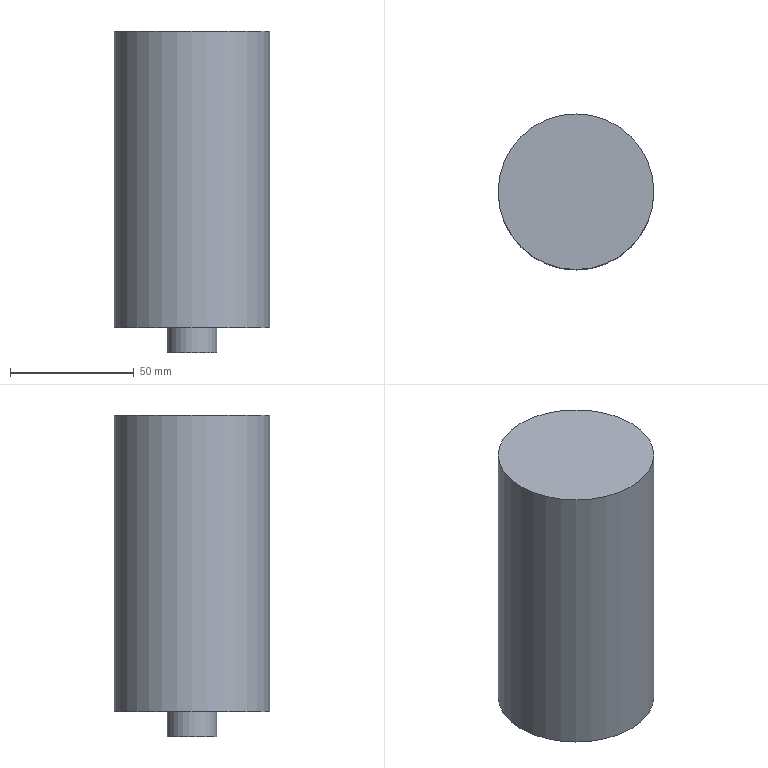Part | NX | features solid 2 | 1 solid | 5 faces | box 63 x 63 x 130 mm | volume 377211 mm3 | plane 3 | cylinder 2 | commonest cylinder face diameters 20 x1 63 x1
STEP:
#1=CARTESIAN_POINT('',(-1296.5,520.,50.));
#2=VERTEX_POINT('',#1);
#3=CARTESIAN_POINT('',(-1265.,520.,50.));
#4=DIRECTION('',(0.,0.,-1.));
#5=DIRECTION('',(-1.,0.,0.));
#6=AXIS2_PLACEMENT_3D('',#3,#4,#5);
#7=CIRCLE('',#6,31.5);
#8=EDGE_CURVE('',#2,#2,#7,.F.);
#9=ORIENTED_EDGE('',*,*,#8,.F.);
#10=EDGE_LOOP('',(#9));
#11=FACE_BOUND('',#10,.T.);
#12=CARTESIAN_POINT('',(-1296.5,520.,-70.));
#13=VERTEX_POINT('',#12);
#14=CARTESIAN_POINT('',(-1265.,520.,-70.));
#15=DIRECTION('',(0.,0.,-1.));
#16=DIRECTION('',(-1.,0.,0.));
#17=AXIS2_PLACEMENT_3D('',#14,#15,#16);
#18=CIRCLE('',#17,31.5);
#19=EDGE_CURVE('',#13,#13,#18,.F.);
#20=ORIENTED_EDGE('',*,*,#19,.T.);
#21=EDGE_LOOP('',(#20));
#22=FACE_BOUND('',#21,.T.);
#23=CARTESIAN_POINT('',(-1265.,520.,-20.));
#24=DIRECTION('',(0.,0.,-1.));
#25=DIRECTION('',(0.,1.,0.));
#26=AXIS2_PLACEMENT_3D('',#23,#24,#25);
#27=CYLINDRICAL_SURFACE('',#26,31.5);
#28=ADVANCED_FACE('',(#11,#22),#27,.T.);
#29=ORIENTED_EDGE('',*,*,#8,.T.);
#30=EDGE_LOOP('',(#29));
#31=FACE_BOUND('',#30,.T.);
#32=CARTESIAN_POINT('',(-1265.,520.,50.));
#33=DIRECTION('',(0.,0.,-1.));
#34=DIRECTION('',(0.,1.,0.));
#35=AXIS2_PLACEMENT_3D('',#32,#33,#34);
#36=PLANE('',#35);
#37=ADVANCED_FACE('',(#31),#36,.F.);
#38=CARTESIAN_POINT('',(-1265.,510.,-70.));
#39=VERTEX_POINT('',#38);
#40=CARTESIAN_POINT('',(-1265.,520.,-70.));
#41=DIRECTION('',(0.,0.,1.));
#42=DIRECTION('',(0.,-1.,0.));
#43=AXIS2_PLACEMENT_3D('',#40,#41,#42);
#44=CIRCLE('',#43,10.);
#45=EDGE_CURVE('',#39,#39,#44,.T.);
#46=ORIENTED_EDGE('',*,*,#45,.T.);
#47=EDGE_LOOP('',(#46));
#48=FACE_BOUND('',#47,.T.);
#49=ORIENTED_EDGE('',*,*,#19,.F.);
#50=EDGE_LOOP('',(#49));
#51=FACE_BOUND('',#50,.T.);
#52=CARTESIAN_POINT('',(-1265.,520.,-70.));
#53=DIRECTION('',(0.,0.,-1.));
#54=DIRECTION('',(0.,1.,0.));
#55=AXIS2_PLACEMENT_3D('',#52,#53,#54);
#56=PLANE('',#55);
#57=ADVANCED_FACE('',(#48,#51),#56,.T.);
#58=ORIENTED_EDGE('',*,*,#45,.F.);
#59=EDGE_LOOP('',(#58));
#60=FACE_BOUND('',#59,.T.);
#61=CARTESIAN_POINT('',(-1265.,510.,-80.));
#62=VERTEX_POINT('',#61);
#63=CARTESIAN_POINT('',(-1265.,520.,-80.));
#64=DIRECTION('',(0.,0.,1.));
#65=DIRECTION('',(0.,-1.,0.));
#66=AXIS2_PLACEMENT_3D('',#63,#64,#65);
#67=CIRCLE('',#66,10.);
#68=EDGE_CURVE('',#62,#62,#67,.T.);
#69=ORIENTED_EDGE('',*,*,#68,.T.);
#70=EDGE_LOOP('',(#69));
#71=FACE_BOUND('',#70,.T.);
#72=CARTESIAN_POINT('',(-1265.,520.,-80.));
#73=DIRECTION('',(0.,0.,-1.));
#74=DIRECTION('',(0.,1.,0.));
#75=AXIS2_PLACEMENT_3D('',#72,#73,#74);
#76=CYLINDRICAL_SURFACE('',#75,10.);
#77=ADVANCED_FACE('',(#60,#71),#76,.T.);
#78=ORIENTED_EDGE('',*,*,#68,.F.);
#79=EDGE_LOOP('',(#78));
#80=FACE_BOUND('',#79,.T.);
#81=CARTESIAN_POINT('',(-1265.,520.,-80.));
#82=DIRECTION('',(0.,0.,-1.));
#83=DIRECTION('',(0.,1.,0.));
#84=AXIS2_PLACEMENT_3D('',#81,#82,#83);
#85=PLANE('',#84);
#86=ADVANCED_FACE('',(#80),#85,.T.);
#87=CLOSED_SHELL('',(#28,#37,#57,#77,#86));
#88=MANIFOLD_SOLID_BREP('',#87);
#89=(LENGTH_UNIT()NAMED_UNIT(*)SI_UNIT(.MILLI.,.METRE.));
#90=UNCERTAINTY_MEASURE_WITH_UNIT(LENGTH_MEASURE(0.00001),#89,'','');
#91=(NAMED_UNIT(*)PLANE_ANGLE_UNIT()SI_UNIT($,.RADIAN.));
#92=(NAMED_UNIT(*)SI_UNIT($,.STERADIAN.)SOLID_ANGLE_UNIT());
#93=(GEOMETRIC_REPRESENTATION_CONTEXT(3)GLOBAL_UNCERTAINTY_ASSIGNED_CONTEXT((#90))GLOBAL_UNIT_ASSIGNED_CONTEXT((#89,#91,#92))REPRESENTATION_CONTEXT('',''));
#94=ADVANCED_BREP_SHAPE_REPRESENTATION('',(#88),#93);